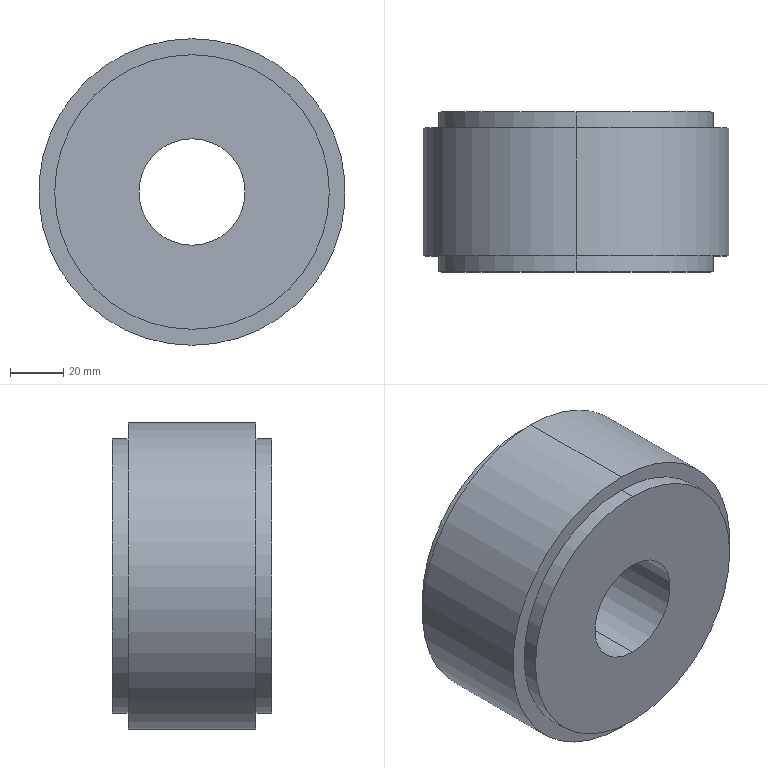Part | SolidWorks | features Revolution 1 | 1 solid | 12 faces | box 115 x 60 x 115 mm | volume 523160 mm3 | cylinder 8 | plane 4 | commonest cylinder face diameters 103 x4 40 x2 115 x2
STEP:
#1=CARTESIAN_POINT('',(0.,3.767,51.5));
#2=VERTEX_POINT('',#1);
#3=CARTESIAN_POINT('',(0.,3.767,-51.5));
#4=VERTEX_POINT('',#3);
#5=CARTESIAN_POINT('',(0.,3.767,0.));
#6=DIRECTION('',(0.,1.,0.));
#7=DIRECTION('',(0.,0.,1.));
#8=AXIS2_PLACEMENT_3D('',#5,#6,#7);
#9=CIRCLE('',#8,51.5);
#10=EDGE_CURVE('',#2,#4,#9,.T.);
#11=ORIENTED_EDGE('',*,*,#10,.T.);
#12=CARTESIAN_POINT('',(0.,9.767,-51.5));
#13=VERTEX_POINT('',#12);
#14=CARTESIAN_POINT('',(0.,27.589,-51.5));
#15=DIRECTION('',(0.,1.,0.));
#16=VECTOR('',#15,1000.);
#17=LINE('',#14,#16);
#18=EDGE_CURVE('',#4,#13,#17,.T.);
#19=ORIENTED_EDGE('',*,*,#18,.T.);
#20=CARTESIAN_POINT('',(0.,9.767,51.5));
#21=VERTEX_POINT('',#20);
#22=CARTESIAN_POINT('',(0.,9.767,0.));
#23=DIRECTION('',(0.,1.,0.));
#24=DIRECTION('',(0.,0.,1.));
#25=AXIS2_PLACEMENT_3D('',#22,#23,#24);
#26=CIRCLE('',#25,51.5);
#27=EDGE_CURVE('',#21,#13,#26,.T.);
#28=ORIENTED_EDGE('',*,*,#27,.F.);
#29=CARTESIAN_POINT('',(0.,27.589,51.5));
#30=DIRECTION('',(0.,1.,0.));
#31=VECTOR('',#30,1000.);
#32=LINE('',#29,#31);
#33=EDGE_CURVE('',#2,#21,#32,.T.);
#34=ORIENTED_EDGE('',*,*,#33,.F.);
#35=EDGE_LOOP('',(#11,#19,#28,#34));
#36=FACE_OUTER_BOUND('',#35,.T.);
#37=CARTESIAN_POINT('',(0.,27.589,0.));
#38=DIRECTION('',(0.,1.,0.));
#39=DIRECTION('',(0.,0.,1.));
#40=AXIS2_PLACEMENT_3D('',#37,#38,#39);
#41=CYLINDRICAL_SURFACE('',#40,51.5);
#42=ADVANCED_FACE('',(#36),#41,.T.);
#43=CARTESIAN_POINT('',(0.,-44.233,57.5));
#44=VERTEX_POINT('',#43);
#45=CARTESIAN_POINT('',(0.,-44.233,-57.5));
#46=VERTEX_POINT('',#45);
#47=CARTESIAN_POINT('',(0.,-44.233,0.));
#48=DIRECTION('',(0.,1.,0.));
#49=DIRECTION('',(0.,0.,1.));
#50=AXIS2_PLACEMENT_3D('',#47,#48,#49);
#51=CIRCLE('',#50,57.5);
#52=EDGE_CURVE('',#44,#46,#51,.T.);
#53=ORIENTED_EDGE('',*,*,#52,.T.);
#54=CARTESIAN_POINT('',(0.,3.767,-57.5));
#55=VERTEX_POINT('',#54);
#56=CARTESIAN_POINT('',(0.,27.589,-57.5));
#57=DIRECTION('',(0.,1.,0.));
#58=VECTOR('',#57,1000.);
#59=LINE('',#56,#58);
#60=EDGE_CURVE('',#46,#55,#59,.T.);
#61=ORIENTED_EDGE('',*,*,#60,.T.);
#62=CARTESIAN_POINT('',(0.,3.767,57.5));
#63=VERTEX_POINT('',#62);
#64=CARTESIAN_POINT('',(0.,3.767,0.));
#65=DIRECTION('',(0.,1.,0.));
#66=DIRECTION('',(0.,0.,1.));
#67=AXIS2_PLACEMENT_3D('',#64,#65,#66);
#68=CIRCLE('',#67,57.5);
#69=EDGE_CURVE('',#63,#55,#68,.T.);
#70=ORIENTED_EDGE('',*,*,#69,.F.);
#71=CARTESIAN_POINT('',(0.,27.589,57.5));
#72=DIRECTION('',(0.,1.,0.));
#73=VECTOR('',#72,1000.);
#74=LINE('',#71,#73);
#75=EDGE_CURVE('',#44,#63,#74,.T.);
#76=ORIENTED_EDGE('',*,*,#75,.F.);
#77=EDGE_LOOP('',(#53,#61,#70,#76));
#78=FACE_OUTER_BOUND('',#77,.T.);
#79=CARTESIAN_POINT('',(0.,27.589,0.));
#80=DIRECTION('',(0.,1.,0.));
#81=DIRECTION('',(0.,0.,1.));
#82=AXIS2_PLACEMENT_3D('',#79,#80,#81);
#83=CYLINDRICAL_SURFACE('',#82,57.5);
#84=ADVANCED_FACE('',(#78),#83,.T.);
#85=CARTESIAN_POINT('',(0.,-50.233,51.5));
#86=VERTEX_POINT('',#85);
#87=CARTESIAN_POINT('',(0.,-50.233,-51.5));
#88=VERTEX_POINT('',#87);
#89=CARTESIAN_POINT('',(0.,-50.233,0.));
#90=DIRECTION('',(0.,1.,0.));
#91=DIRECTION('',(0.,0.,1.));
#92=AXIS2_PLACEMENT_3D('',#89,#90,#91);
#93=CIRCLE('',#92,51.5);
#94=EDGE_CURVE('',#86,#88,#93,.T.);
#95=ORIENTED_EDGE('',*,*,#94,.T.);
#96=CARTESIAN_POINT('',(0.,-44.233,-51.5));
#97=VERTEX_POINT('',#96);
#98=CARTESIAN_POINT('',(0.,27.589,-51.5));
#99=DIRECTION('',(0.,1.,0.));
#100=VECTOR('',#99,1000.);
#101=LINE('',#98,#100);
#102=EDGE_CURVE('',#88,#97,#101,.T.);
#103=ORIENTED_EDGE('',*,*,#102,.T.);
#104=CARTESIAN_POINT('',(0.,-44.233,51.5));
#105=VERTEX_POINT('',#104);
#106=CARTESIAN_POINT('',(0.,-44.233,0.));
#107=DIRECTION('',(0.,1.,0.));
#108=DIRECTION('',(0.,0.,1.));
#109=AXIS2_PLACEMENT_3D('',#106,#107,#108);
#110=CIRCLE('',#109,51.5);
#111=EDGE_CURVE('',#105,#97,#110,.T.);
#112=ORIENTED_EDGE('',*,*,#111,.F.);
#113=CARTESIAN_POINT('',(0.,27.589,51.5));
#114=DIRECTION('',(0.,1.,0.));
#115=VECTOR('',#114,1000.);
#116=LINE('',#113,#115);
#117=EDGE_CURVE('',#86,#105,#116,.T.);
#118=ORIENTED_EDGE('',*,*,#117,.F.);
#119=EDGE_LOOP('',(#95,#103,#112,#118));
#120=FACE_OUTER_BOUND('',#119,.T.);
#121=CARTESIAN_POINT('',(0.,27.589,0.));
#122=DIRECTION('',(0.,1.,0.));
#123=DIRECTION('',(0.,0.,1.));
#124=AXIS2_PLACEMENT_3D('',#121,#122,#123);
#125=CYLINDRICAL_SURFACE('',#124,51.5);
#126=ADVANCED_FACE('',(#120),#125,.T.);
#127=CARTESIAN_POINT('',(0.,-50.233,-20.));
#128=VERTEX_POINT('',#127);
#129=CARTESIAN_POINT('',(0.,-50.233,20.));
#130=VERTEX_POINT('',#129);
#131=CARTESIAN_POINT('',(0.,-50.233,0.));
#132=DIRECTION('',(0.,1.,0.));
#133=DIRECTION('',(0.,0.,1.));
#134=AXIS2_PLACEMENT_3D('',#131,#132,#133);
#135=CIRCLE('',#134,20.);
#136=EDGE_CURVE('',#128,#130,#135,.T.);
#137=ORIENTED_EDGE('',*,*,#136,.F.);
#138=CARTESIAN_POINT('',(0.,9.767,-20.));
#139=VERTEX_POINT('',#138);
#140=CARTESIAN_POINT('',(0.,27.589,-20.));
#141=DIRECTION('',(0.,1.,0.));
#142=VECTOR('',#141,1000.);
#143=LINE('',#140,#142);
#144=EDGE_CURVE('',#128,#139,#143,.T.);
#145=ORIENTED_EDGE('',*,*,#144,.T.);
#146=CARTESIAN_POINT('',(0.,9.767,20.));
#147=VERTEX_POINT('',#146);
#148=CARTESIAN_POINT('',(0.,9.767,0.));
#149=DIRECTION('',(0.,1.,0.));
#150=DIRECTION('',(0.,0.,1.));
#151=AXIS2_PLACEMENT_3D('',#148,#149,#150);
#152=CIRCLE('',#151,20.);
#153=EDGE_CURVE('',#139,#147,#152,.T.);
#154=ORIENTED_EDGE('',*,*,#153,.T.);
#155=CARTESIAN_POINT('',(0.,27.589,20.));
#156=DIRECTION('',(0.,1.,0.));
#157=VECTOR('',#156,1000.);
#158=LINE('',#155,#157);
#159=EDGE_CURVE('',#130,#147,#158,.T.);
#160=ORIENTED_EDGE('',*,*,#159,.F.);
#161=EDGE_LOOP('',(#137,#145,#154,#160));
#162=FACE_OUTER_BOUND('',#161,.T.);
#163=CARTESIAN_POINT('',(0.,27.589,0.));
#164=DIRECTION('',(0.,1.,0.));
#165=DIRECTION('',(0.,0.,1.));
#166=AXIS2_PLACEMENT_3D('',#163,#164,#165);
#167=CYLINDRICAL_SURFACE('',#166,20.);
#168=ADVANCED_FACE('',(#162),#167,.F.);
#169=CARTESIAN_POINT('',(0.,9.767,0.));
#170=DIRECTION('',(0.,1.,0.));
#171=DIRECTION('',(0.,0.,1.));
#172=AXIS2_PLACEMENT_3D('',#169,#170,#171);
#173=CIRCLE('',#172,20.);
#174=EDGE_CURVE('',#147,#139,#173,.T.);
#175=ORIENTED_EDGE('',*,*,#174,.F.);
#176=ORIENTED_EDGE('',*,*,#153,.F.);
#177=EDGE_LOOP('',(#175,#176));
#178=FACE_BOUND('',#177,.T.);
#179=ORIENTED_EDGE('',*,*,#27,.T.);
#180=CARTESIAN_POINT('',(0.,9.767,0.));
#181=DIRECTION('',(0.,1.,0.));
#182=DIRECTION('',(0.,0.,1.));
#183=AXIS2_PLACEMENT_3D('',#180,#181,#182);
#184=CIRCLE('',#183,51.5);
#185=EDGE_CURVE('',#13,#21,#184,.T.);
#186=ORIENTED_EDGE('',*,*,#185,.T.);
#187=EDGE_LOOP('',(#179,#186));
#188=FACE_OUTER_BOUND('',#187,.T.);
#189=CARTESIAN_POINT('',(51.5,9.767,0.));
#190=DIRECTION('',(0.,-1.,0.));
#191=DIRECTION('',(0.,0.,-1.));
#192=AXIS2_PLACEMENT_3D('',#189,#190,#191);
#193=PLANE('',#192);
#194=ADVANCED_FACE('',(#178,#188),#193,.F.);
#195=ORIENTED_EDGE('',*,*,#144,.F.);
#196=CARTESIAN_POINT('',(0.,-50.233,0.));
#197=DIRECTION('',(0.,1.,0.));
#198=DIRECTION('',(0.,0.,1.));
#199=AXIS2_PLACEMENT_3D('',#196,#197,#198);
#200=CIRCLE('',#199,20.);
#201=EDGE_CURVE('',#130,#128,#200,.T.);
#202=ORIENTED_EDGE('',*,*,#201,.F.);
#203=ORIENTED_EDGE('',*,*,#159,.T.);
#204=ORIENTED_EDGE('',*,*,#174,.T.);
#205=EDGE_LOOP('',(#195,#202,#203,#204));
#206=FACE_OUTER_BOUND('',#205,.T.);
#207=CARTESIAN_POINT('',(0.,27.589,0.));
#208=DIRECTION('',(0.,1.,0.));
#209=DIRECTION('',(0.,0.,1.));
#210=AXIS2_PLACEMENT_3D('',#207,#208,#209);
#211=CYLINDRICAL_SURFACE('',#210,20.);
#212=ADVANCED_FACE('',(#206),#211,.F.);
#213=ORIENTED_EDGE('',*,*,#94,.F.);
#214=CARTESIAN_POINT('',(0.,-50.233,0.));
#215=DIRECTION('',(0.,1.,0.));
#216=DIRECTION('',(0.,0.,1.));
#217=AXIS2_PLACEMENT_3D('',#214,#215,#216);
#218=CIRCLE('',#217,51.5);
#219=EDGE_CURVE('',#88,#86,#218,.T.);
#220=ORIENTED_EDGE('',*,*,#219,.F.);
#221=EDGE_LOOP('',(#213,#220));
#222=FACE_OUTER_BOUND('',#221,.T.);
#223=ORIENTED_EDGE('',*,*,#201,.T.);
#224=ORIENTED_EDGE('',*,*,#136,.T.);
#225=EDGE_LOOP('',(#223,#224));
#226=FACE_BOUND('',#225,.T.);
#227=CARTESIAN_POINT('',(20.,-50.233,0.));
#228=DIRECTION('',(0.,1.,0.));
#229=DIRECTION('',(0.,0.,1.));
#230=AXIS2_PLACEMENT_3D('',#227,#228,#229);
#231=PLANE('',#230);
#232=ADVANCED_FACE('',(#222,#226),#231,.F.);
#233=ORIENTED_EDGE('',*,*,#102,.F.);
#234=ORIENTED_EDGE('',*,*,#219,.T.);
#235=ORIENTED_EDGE('',*,*,#117,.T.);
#236=CARTESIAN_POINT('',(0.,-44.233,0.));
#237=DIRECTION('',(0.,1.,0.));
#238=DIRECTION('',(0.,0.,1.));
#239=AXIS2_PLACEMENT_3D('',#236,#237,#238);
#240=CIRCLE('',#239,51.5);
#241=EDGE_CURVE('',#97,#105,#240,.T.);
#242=ORIENTED_EDGE('',*,*,#241,.F.);
#243=EDGE_LOOP('',(#233,#234,#235,#242));
#244=FACE_OUTER_BOUND('',#243,.T.);
#245=CARTESIAN_POINT('',(0.,27.589,0.));
#246=DIRECTION('',(0.,1.,0.));
#247=DIRECTION('',(0.,0.,1.));
#248=AXIS2_PLACEMENT_3D('',#245,#246,#247);
#249=CYLINDRICAL_SURFACE('',#248,51.5);
#250=ADVANCED_FACE('',(#244),#249,.T.);
#251=ORIENTED_EDGE('',*,*,#52,.F.);
#252=CARTESIAN_POINT('',(0.,-44.233,0.));
#253=DIRECTION('',(0.,1.,0.));
#254=DIRECTION('',(0.,0.,1.));
#255=AXIS2_PLACEMENT_3D('',#252,#253,#254);
#256=CIRCLE('',#255,57.5);
#257=EDGE_CURVE('',#46,#44,#256,.T.);
#258=ORIENTED_EDGE('',*,*,#257,.F.);
#259=EDGE_LOOP('',(#251,#258));
#260=FACE_OUTER_BOUND('',#259,.T.);
#261=ORIENTED_EDGE('',*,*,#111,.T.);
#262=ORIENTED_EDGE('',*,*,#241,.T.);
#263=EDGE_LOOP('',(#261,#262));
#264=FACE_BOUND('',#263,.T.);
#265=CARTESIAN_POINT('',(51.5,-44.233,0.));
#266=DIRECTION('',(0.,1.,0.));
#267=DIRECTION('',(0.,0.,1.));
#268=AXIS2_PLACEMENT_3D('',#265,#266,#267);
#269=PLANE('',#268);
#270=ADVANCED_FACE('',(#260,#264),#269,.F.);
#271=ORIENTED_EDGE('',*,*,#60,.F.);
#272=ORIENTED_EDGE('',*,*,#257,.T.);
#273=ORIENTED_EDGE('',*,*,#75,.T.);
#274=CARTESIAN_POINT('',(0.,3.767,0.));
#275=DIRECTION('',(0.,1.,0.));
#276=DIRECTION('',(0.,0.,1.));
#277=AXIS2_PLACEMENT_3D('',#274,#275,#276);
#278=CIRCLE('',#277,57.5);
#279=EDGE_CURVE('',#55,#63,#278,.T.);
#280=ORIENTED_EDGE('',*,*,#279,.F.);
#281=EDGE_LOOP('',(#271,#272,#273,#280));
#282=FACE_OUTER_BOUND('',#281,.T.);
#283=CARTESIAN_POINT('',(0.,27.589,0.));
#284=DIRECTION('',(0.,1.,0.));
#285=DIRECTION('',(0.,0.,1.));
#286=AXIS2_PLACEMENT_3D('',#283,#284,#285);
#287=CYLINDRICAL_SURFACE('',#286,57.5);
#288=ADVANCED_FACE('',(#282),#287,.T.);
#289=ORIENTED_EDGE('',*,*,#10,.F.);
#290=CARTESIAN_POINT('',(0.,3.767,0.));
#291=DIRECTION('',(0.,1.,0.));
#292=DIRECTION('',(0.,0.,1.));
#293=AXIS2_PLACEMENT_3D('',#290,#291,#292);
#294=CIRCLE('',#293,51.5);
#295=EDGE_CURVE('',#4,#2,#294,.T.);
#296=ORIENTED_EDGE('',*,*,#295,.F.);
#297=EDGE_LOOP('',(#289,#296));
#298=FACE_BOUND('',#297,.T.);
#299=ORIENTED_EDGE('',*,*,#69,.T.);
#300=ORIENTED_EDGE('',*,*,#279,.T.);
#301=EDGE_LOOP('',(#299,#300));
#302=FACE_OUTER_BOUND('',#301,.T.);
#303=CARTESIAN_POINT('',(57.5,3.767,0.));
#304=DIRECTION('',(0.,-1.,0.));
#305=DIRECTION('',(0.,0.,-1.));
#306=AXIS2_PLACEMENT_3D('',#303,#304,#305);
#307=PLANE('',#306);
#308=ADVANCED_FACE('',(#298,#302),#307,.F.);
#309=ORIENTED_EDGE('',*,*,#18,.F.);
#310=ORIENTED_EDGE('',*,*,#295,.T.);
#311=ORIENTED_EDGE('',*,*,#33,.T.);
#312=ORIENTED_EDGE('',*,*,#185,.F.);
#313=EDGE_LOOP('',(#309,#310,#311,#312));
#314=FACE_OUTER_BOUND('',#313,.T.);
#315=CARTESIAN_POINT('',(0.,27.589,0.));
#316=DIRECTION('',(0.,1.,0.));
#317=DIRECTION('',(0.,0.,1.));
#318=AXIS2_PLACEMENT_3D('',#315,#316,#317);
#319=CYLINDRICAL_SURFACE('',#318,51.5);
#320=ADVANCED_FACE('',(#314),#319,.T.);
#321=CLOSED_SHELL('',(#42,#84,#126,#168,#194,#212,#232,#250,#270,#288,#308,#320));
#322=MANIFOLD_SOLID_BREP('',#321);
#323=CARTESIAN_POINT('',(0.,0.,0.));
#324=DIRECTION('',(0.,0.,1.));
#325=DIRECTION('',(1.,0.,0.));
#326=AXIS2_PLACEMENT_3D('',#323,#324,#325);
#327=(LENGTH_UNIT()NAMED_UNIT(*)SI_UNIT(.MILLI.,.METRE.));
#328=UNCERTAINTY_MEASURE_WITH_UNIT(LENGTH_MEASURE(0.00001),#327,'','');
#329=(NAMED_UNIT(*)PLANE_ANGLE_UNIT()SI_UNIT($,.RADIAN.));
#330=(NAMED_UNIT(*)SI_UNIT($,.STERADIAN.)SOLID_ANGLE_UNIT());
#331=(GEOMETRIC_REPRESENTATION_CONTEXT(3)GLOBAL_UNCERTAINTY_ASSIGNED_CONTEXT((#328))GLOBAL_UNIT_ASSIGNED_CONTEXT((#327,#329,#330))REPRESENTATION_CONTEXT('',''));
#332=ADVANCED_BREP_SHAPE_REPRESENTATION('',(#322,#326),#331);